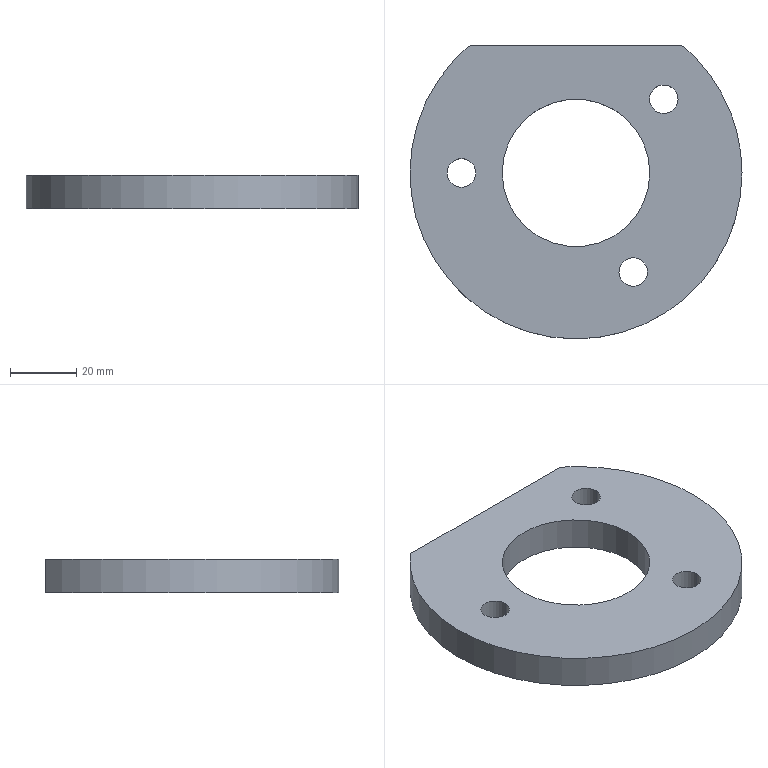Part | STEP file | 1_id1230_x_t | 1 solid | 12 faces | box 100 x 88.5 x 10 mm | volume 56263 mm3 | cylinder 9 | plane 3 | commonest cylinder face diameters 8.6 x6 44.45 x2 100 x1
STEP:
#1=CARTESIAN_POINT('',(0.,0.,0.));
#2=DIRECTION('',(0.,0.,1.));
#3=DIRECTION('',(1.,0.,0.));
#4=AXIS2_PLACEMENT_3D('',#1,#2,#3);
#5=CARTESIAN_POINT('',(112.925,347.5,90.11));
#6=VERTEX_POINT('',#5);
#7=CARTESIAN_POINT('',(31.023,386.,90.11));
#8=VERTEX_POINT('',#7);
#9=CARTESIAN_POINT('',(62.925,347.5,90.11));
#10=DIRECTION('',(0.,0.,-1.));
#11=DIRECTION('',(1.,0.,0.));
#12=AXIS2_PLACEMENT_3D('',#9,#10,#11);
#13=CIRCLE('',#12,50.);
#14=CARTESIAN_POINT('',(62.925,347.5,90.11));
#15=DIRECTION('',(0.,0.,1.));
#16=DIRECTION('',(1.,0.,0.));
#17=AXIS2_PLACEMENT_3D('',#14,#15,#16);
#18=PLANE('',#17);
#19=CARTESIAN_POINT('',(50.,0.));
#20=CARTESIAN_POINT('',(50.,-86.603));
#21=CARTESIAN_POINT('',(-25.,-43.301));
#22=CARTESIAN_POINT('',(-100.,0.));
#23=CARTESIAN_POINT('',(-25.,43.301));
#24=CARTESIAN_POINT('',(50.,86.603));
#25=CARTESIAN_POINT('',(50.,0.));
#26=(BOUNDED_CURVE()B_SPLINE_CURVE(2,(#19,#20,#21,#22,#23,#24,#25),.UNSPECIFIED.,.T.,.F.)B_SPLINE_CURVE_WITH_KNOTS((1,2,2,2,2,1),(-2.094,0.,2.094,4.189,6.283,8.378),.UNSPECIFIED.)CURVE()GEOMETRIC_REPRESENTATION_ITEM()RATIONAL_B_SPLINE_CURVE((1.,0.5,1.,0.5,1.,0.5,1.))REPRESENTATION_ITEM(''));
#27=(GEOMETRIC_REPRESENTATION_CONTEXT(2)PARAMETRIC_REPRESENTATION_CONTEXT()REPRESENTATION_CONTEXT('',''));
#28=DEFINITIONAL_REPRESENTATION('',(#26),#27);
#29=PCURVE('',#18,#28);
#30=CARTESIAN_POINT('',(62.925,347.5,100.11));
#31=DIRECTION('',(0.,0.,-1.));
#32=DIRECTION('',(-1.,0.,0.));
#33=AXIS2_PLACEMENT_3D('',#30,#31,#32);
#34=CYLINDRICAL_SURFACE('',#33,50.);
#35=CARTESIAN_POINT('',(3.142,10.));
#36=DIRECTION('',(1.,0.));
#37=VECTOR('',#36,1.);
#38=LINE('',#35,#37);
#39=(GEOMETRIC_REPRESENTATION_CONTEXT(2)PARAMETRIC_REPRESENTATION_CONTEXT()REPRESENTATION_CONTEXT('',''));
#40=DEFINITIONAL_REPRESENTATION('',(#38),#39);
#41=PCURVE('',#34,#40);
#42=SURFACE_CURVE('',#13,(#29,#41),.PCURVE_S1.);
#43=EDGE_CURVE('',#6,#8,#42,.T.);
#44=ORIENTED_EDGE('',*,*,#43,.T.);
#45=CARTESIAN_POINT('',(94.827,386.,90.11));
#46=VERTEX_POINT('',#45);
#47=CARTESIAN_POINT('',(94.827,386.,90.11));
#48=DIRECTION('',(-1.,0.,0.));
#49=VECTOR('',#48,1.);
#50=LINE('',#47,#49);
#51=CARTESIAN_POINT('',(31.902,38.5));
#52=DIRECTION('',(-1.,0.));
#53=VECTOR('',#52,1.);
#54=LINE('',#51,#53);
#55=(GEOMETRIC_REPRESENTATION_CONTEXT(2)PARAMETRIC_REPRESENTATION_CONTEXT()REPRESENTATION_CONTEXT('',''));
#56=DEFINITIONAL_REPRESENTATION('',(#54),#55);
#57=PCURVE('',#18,#56);
#58=CARTESIAN_POINT('',(167.925,386.,-58.465));
#59=DIRECTION('',(0.,-1.,0.));
#60=DIRECTION('',(0.,0.,1.));
#61=AXIS2_PLACEMENT_3D('',#58,#59,#60);
#62=PLANE('',#61);
#63=CARTESIAN_POINT('',(148.575,73.098));
#64=DIRECTION('',(0.,1.));
#65=VECTOR('',#64,1.);
#66=LINE('',#63,#65);
#67=(GEOMETRIC_REPRESENTATION_CONTEXT(2)PARAMETRIC_REPRESENTATION_CONTEXT()REPRESENTATION_CONTEXT('',''));
#68=DEFINITIONAL_REPRESENTATION('',(#66),#67);
#69=PCURVE('',#62,#68);
#70=SURFACE_CURVE('',#50,(#57,#69),.PCURVE_S1.);
#71=EDGE_CURVE('',#46,#8,#70,.T.);
#72=ORIENTED_EDGE('',*,*,#71,.F.);
#73=CARTESIAN_POINT('',(62.925,347.5,90.11));
#74=DIRECTION('',(0.,0.,-1.));
#75=DIRECTION('',(0.638,0.77,0.));
#76=AXIS2_PLACEMENT_3D('',#73,#74,#75);
#77=CIRCLE('',#76,50.);
#78=CARTESIAN_POINT('',(31.902,38.5));
#79=CARTESIAN_POINT('',(98.586,-16.756));
#80=CARTESIAN_POINT('',(17.391,-46.878));
#81=CARTESIAN_POINT('',(-63.804,-77.));
#82=CARTESIAN_POINT('',(-49.293,8.378));
#83=CARTESIAN_POINT('',(-34.782,93.756));
#84=CARTESIAN_POINT('',(31.902,38.5));
#85=(BOUNDED_CURVE()B_SPLINE_CURVE(2,(#78,#79,#80,#81,#82,#83,#84),.UNSPECIFIED.,.T.,.F.)B_SPLINE_CURVE_WITH_KNOTS((1,2,2,2,2,1),(-2.094,0.,2.094,4.189,6.283,8.378),.UNSPECIFIED.)CURVE()GEOMETRIC_REPRESENTATION_ITEM()RATIONAL_B_SPLINE_CURVE((1.,0.5,1.,0.5,1.,0.5,1.))REPRESENTATION_ITEM(''));
#86=(GEOMETRIC_REPRESENTATION_CONTEXT(2)PARAMETRIC_REPRESENTATION_CONTEXT()REPRESENTATION_CONTEXT('',''));
#87=DEFINITIONAL_REPRESENTATION('',(#85),#86);
#88=PCURVE('',#18,#87);
#89=CARTESIAN_POINT('',(2.263,10.));
#90=DIRECTION('',(1.,0.));
#91=VECTOR('',#90,1.);
#92=LINE('',#89,#91);
#93=(GEOMETRIC_REPRESENTATION_CONTEXT(2)PARAMETRIC_REPRESENTATION_CONTEXT()REPRESENTATION_CONTEXT('',''));
#94=DEFINITIONAL_REPRESENTATION('',(#92),#93);
#95=PCURVE('',#34,#94);
#96=SURFACE_CURVE('',#77,(#88,#95),.PCURVE_S1.);
#97=EDGE_CURVE('',#46,#6,#96,.T.);
#98=ORIENTED_EDGE('',*,*,#97,.T.);
#99=EDGE_LOOP('',(#44,#72,#98));
#100=FACE_BOUND('',#99,.T.);
#101=CARTESIAN_POINT('',(74.037,328.253,90.11));
#102=VERTEX_POINT('',#101);
#103=CARTESIAN_POINT('',(51.812,366.747,90.11));
#104=VERTEX_POINT('',#103);
#105=CARTESIAN_POINT('',(62.925,347.5,90.11));
#106=DIRECTION('',(0.,0.,1.));
#107=DIRECTION('',(0.5,-0.866,0.));
#108=AXIS2_PLACEMENT_3D('',#105,#106,#107);
#109=CIRCLE('',#108,22.225);
#110=CARTESIAN_POINT('',(0.,0.));
#111=DIRECTION('',(0.5,-0.866));
#112=AXIS2_PLACEMENT_2D('',#110,#111);
#113=CIRCLE('',#112,22.225);
#114=(GEOMETRIC_REPRESENTATION_CONTEXT(2)PARAMETRIC_REPRESENTATION_CONTEXT()REPRESENTATION_CONTEXT('',''));
#115=DEFINITIONAL_REPRESENTATION('',(#113),#114);
#116=PCURVE('',#18,#115);
#117=CARTESIAN_POINT('',(62.925,347.5,91.735));
#118=DIRECTION('',(0.,0.,1.));
#119=DIRECTION('',(-0.5,0.866,0.));
#120=AXIS2_PLACEMENT_3D('',#117,#118,#119);
#121=CYLINDRICAL_SURFACE('',#120,22.225);
#122=CARTESIAN_POINT('',(3.142,-1.625));
#123=DIRECTION('',(1.,0.));
#124=VECTOR('',#123,1.);
#125=LINE('',#122,#124);
#126=(GEOMETRIC_REPRESENTATION_CONTEXT(2)PARAMETRIC_REPRESENTATION_CONTEXT()REPRESENTATION_CONTEXT('',''));
#127=DEFINITIONAL_REPRESENTATION('',(#125),#126);
#128=PCURVE('',#121,#127);
#129=SURFACE_CURVE('',#109,(#116,#128),.PCURVE_S1.);
#130=EDGE_CURVE('',#102,#104,#129,.T.);
#131=ORIENTED_EDGE('',*,*,#130,.T.);
#132=CARTESIAN_POINT('',(40.7,347.5,90.11));
#133=VERTEX_POINT('',#132);
#134=CARTESIAN_POINT('',(62.925,347.5,90.11));
#135=DIRECTION('',(0.,0.,1.));
#136=DIRECTION('',(-0.5,0.866,0.));
#137=AXIS2_PLACEMENT_3D('',#134,#135,#136);
#138=CIRCLE('',#137,22.225);
#139=CARTESIAN_POINT('',(0.,0.));
#140=DIRECTION('',(-0.5,0.866));
#141=AXIS2_PLACEMENT_2D('',#139,#140);
#142=CIRCLE('',#141,22.225);
#143=(GEOMETRIC_REPRESENTATION_CONTEXT(2)PARAMETRIC_REPRESENTATION_CONTEXT()REPRESENTATION_CONTEXT('',''));
#144=DEFINITIONAL_REPRESENTATION('',(#142),#143);
#145=PCURVE('',#18,#144);
#146=CARTESIAN_POINT('',(62.925,347.5,91.735));
#147=DIRECTION('',(0.,0.,1.));
#148=DIRECTION('',(-0.5,0.866,0.));
#149=AXIS2_PLACEMENT_3D('',#146,#147,#148);
#150=CYLINDRICAL_SURFACE('',#149,22.225);
#151=CARTESIAN_POINT('',(0.,-1.625));
#152=DIRECTION('',(1.,0.));
#153=VECTOR('',#152,1.);
#154=LINE('',#151,#153);
#155=(GEOMETRIC_REPRESENTATION_CONTEXT(2)PARAMETRIC_REPRESENTATION_CONTEXT()REPRESENTATION_CONTEXT('',''));
#156=DEFINITIONAL_REPRESENTATION('',(#154),#155);
#157=PCURVE('',#150,#156);
#158=SURFACE_CURVE('',#138,(#145,#157),.PCURVE_S1.);
#159=EDGE_CURVE('',#104,#133,#158,.T.);
#160=ORIENTED_EDGE('',*,*,#159,.T.);
#161=CARTESIAN_POINT('',(62.925,347.5,90.11));
#162=DIRECTION('',(0.,0.,1.));
#163=DIRECTION('',(-1.,0.,0.));
#164=AXIS2_PLACEMENT_3D('',#161,#162,#163);
#165=CIRCLE('',#164,22.225);
#166=CARTESIAN_POINT('',(0.,0.));
#167=DIRECTION('',(-1.,0.));
#168=AXIS2_PLACEMENT_2D('',#166,#167);
#169=CIRCLE('',#168,22.225);
#170=(GEOMETRIC_REPRESENTATION_CONTEXT(2)PARAMETRIC_REPRESENTATION_CONTEXT()REPRESENTATION_CONTEXT('',''));
#171=DEFINITIONAL_REPRESENTATION('',(#169),#170);
#172=PCURVE('',#18,#171);
#173=CARTESIAN_POINT('',(1.047,-1.625));
#174=DIRECTION('',(1.,0.));
#175=VECTOR('',#174,1.);
#176=LINE('',#173,#175);
#177=(GEOMETRIC_REPRESENTATION_CONTEXT(2)PARAMETRIC_REPRESENTATION_CONTEXT()REPRESENTATION_CONTEXT('',''));
#178=DEFINITIONAL_REPRESENTATION('',(#176),#177);
#179=PCURVE('',#150,#178);
#180=SURFACE_CURVE('',#165,(#172,#179),.PCURVE_S1.);
#181=EDGE_CURVE('',#133,#102,#180,.T.);
#182=ORIENTED_EDGE('',*,*,#181,.T.);
#183=EDGE_LOOP('',(#131,#160,#182));
#184=FACE_BOUND('',#183,.T.);
#185=CARTESIAN_POINT('',(32.725,347.5,90.11));
#186=VERTEX_POINT('',#185);
#187=CARTESIAN_POINT('',(24.125,347.5,90.11));
#188=VERTEX_POINT('',#187);
#189=CARTESIAN_POINT('',(28.425,347.5,90.11));
#190=DIRECTION('',(0.,0.,1.));
#191=DIRECTION('',(1.,0.,0.));
#192=AXIS2_PLACEMENT_3D('',#189,#190,#191);
#193=CIRCLE('',#192,4.3);
#194=CARTESIAN_POINT('',(-34.5,0.));
#195=DIRECTION('',(1.,0.));
#196=AXIS2_PLACEMENT_2D('',#194,#195);
#197=CIRCLE('',#196,4.3);
#198=(GEOMETRIC_REPRESENTATION_CONTEXT(2)PARAMETRIC_REPRESENTATION_CONTEXT()REPRESENTATION_CONTEXT('',''));
#199=DEFINITIONAL_REPRESENTATION('',(#197),#198);
#200=PCURVE('',#18,#199);
#201=CARTESIAN_POINT('',(28.425,347.5,199.11));
#202=DIRECTION('',(0.,0.,-1.));
#203=DIRECTION('',(-1.,0.,0.));
#204=AXIS2_PLACEMENT_3D('',#201,#202,#203);
#205=CYLINDRICAL_SURFACE('',#204,4.3);
#206=CARTESIAN_POINT('',(3.142,109.));
#207=DIRECTION('',(-1.,0.));
#208=VECTOR('',#207,1.);
#209=LINE('',#206,#208);
#210=(GEOMETRIC_REPRESENTATION_CONTEXT(2)PARAMETRIC_REPRESENTATION_CONTEXT()REPRESENTATION_CONTEXT('',''));
#211=DEFINITIONAL_REPRESENTATION('',(#209),#210);
#212=PCURVE('',#205,#211);
#213=SURFACE_CURVE('',#193,(#200,#212),.PCURVE_S1.);
#214=EDGE_CURVE('',#186,#188,#213,.T.);
#215=ORIENTED_EDGE('',*,*,#214,.T.);
#216=CARTESIAN_POINT('',(28.425,347.5,90.11));
#217=DIRECTION('',(0.,0.,1.));
#218=DIRECTION('',(-1.,0.,0.));
#219=AXIS2_PLACEMENT_3D('',#216,#217,#218);
#220=CIRCLE('',#219,4.3);
#221=CARTESIAN_POINT('',(-34.5,0.));
#222=DIRECTION('',(-1.,0.));
#223=AXIS2_PLACEMENT_2D('',#221,#222);
#224=CIRCLE('',#223,4.3);
#225=(GEOMETRIC_REPRESENTATION_CONTEXT(2)PARAMETRIC_REPRESENTATION_CONTEXT()REPRESENTATION_CONTEXT('',''));
#226=DEFINITIONAL_REPRESENTATION('',(#224),#225);
#227=PCURVE('',#18,#226);
#228=CARTESIAN_POINT('',(28.425,347.5,199.11));
#229=DIRECTION('',(0.,0.,-1.));
#230=DIRECTION('',(-1.,0.,0.));
#231=AXIS2_PLACEMENT_3D('',#228,#229,#230);
#232=CYLINDRICAL_SURFACE('',#231,4.3);
#233=CARTESIAN_POINT('',(6.283,109.));
#234=DIRECTION('',(-1.,0.));
#235=VECTOR('',#234,1.);
#236=LINE('',#233,#235);
#237=(GEOMETRIC_REPRESENTATION_CONTEXT(2)PARAMETRIC_REPRESENTATION_CONTEXT()REPRESENTATION_CONTEXT('',''));
#238=DEFINITIONAL_REPRESENTATION('',(#236),#237);
#239=PCURVE('',#232,#238);
#240=SURFACE_CURVE('',#220,(#227,#239),.PCURVE_S1.);
#241=EDGE_CURVE('',#188,#186,#240,.T.);
#242=ORIENTED_EDGE('',*,*,#241,.T.);
#243=EDGE_LOOP('',(#215,#242));
#244=FACE_BOUND('',#243,.T.);
#245=CARTESIAN_POINT('',(93.654,369.676,90.11));
#246=VERTEX_POINT('',#245);
#247=CARTESIAN_POINT('',(85.054,369.676,90.11));
#248=VERTEX_POINT('',#247);
#249=CARTESIAN_POINT('',(89.354,369.676,90.11));
#250=DIRECTION('',(0.,0.,1.));
#251=DIRECTION('',(1.,0.,0.));
#252=AXIS2_PLACEMENT_3D('',#249,#250,#251);
#253=CIRCLE('',#252,4.3);
#254=CARTESIAN_POINT('',(26.429,22.176));
#255=DIRECTION('',(1.,0.));
#256=AXIS2_PLACEMENT_2D('',#254,#255);
#257=CIRCLE('',#256,4.3);
#258=(GEOMETRIC_REPRESENTATION_CONTEXT(2)PARAMETRIC_REPRESENTATION_CONTEXT()REPRESENTATION_CONTEXT('',''));
#259=DEFINITIONAL_REPRESENTATION('',(#257),#258);
#260=PCURVE('',#18,#259);
#261=CARTESIAN_POINT('',(89.354,369.676,199.11));
#262=DIRECTION('',(0.,0.,-1.));
#263=DIRECTION('',(-1.,0.,0.));
#264=AXIS2_PLACEMENT_3D('',#261,#262,#263);
#265=CYLINDRICAL_SURFACE('',#264,4.3);
#266=CARTESIAN_POINT('',(3.142,109.));
#267=DIRECTION('',(-1.,0.));
#268=VECTOR('',#267,1.);
#269=LINE('',#266,#268);
#270=(GEOMETRIC_REPRESENTATION_CONTEXT(2)PARAMETRIC_REPRESENTATION_CONTEXT()REPRESENTATION_CONTEXT('',''));
#271=DEFINITIONAL_REPRESENTATION('',(#269),#270);
#272=PCURVE('',#265,#271);
#273=SURFACE_CURVE('',#253,(#260,#272),.PCURVE_S1.);
#274=EDGE_CURVE('',#246,#248,#273,.T.);
#275=ORIENTED_EDGE('',*,*,#274,.T.);
#276=CARTESIAN_POINT('',(89.354,369.676,90.11));
#277=DIRECTION('',(0.,0.,1.));
#278=DIRECTION('',(-1.,0.,0.));
#279=AXIS2_PLACEMENT_3D('',#276,#277,#278);
#280=CIRCLE('',#279,4.3);
#281=CARTESIAN_POINT('',(26.429,22.176));
#282=DIRECTION('',(-1.,0.));
#283=AXIS2_PLACEMENT_2D('',#281,#282);
#284=CIRCLE('',#283,4.3);
#285=(GEOMETRIC_REPRESENTATION_CONTEXT(2)PARAMETRIC_REPRESENTATION_CONTEXT()REPRESENTATION_CONTEXT('',''));
#286=DEFINITIONAL_REPRESENTATION('',(#284),#285);
#287=PCURVE('',#18,#286);
#288=CARTESIAN_POINT('',(89.354,369.676,199.11));
#289=DIRECTION('',(0.,0.,-1.));
#290=DIRECTION('',(-1.,0.,0.));
#291=AXIS2_PLACEMENT_3D('',#288,#289,#290);
#292=CYLINDRICAL_SURFACE('',#291,4.3);
#293=CARTESIAN_POINT('',(6.283,109.));
#294=DIRECTION('',(-1.,0.));
#295=VECTOR('',#294,1.);
#296=LINE('',#293,#295);
#297=(GEOMETRIC_REPRESENTATION_CONTEXT(2)PARAMETRIC_REPRESENTATION_CONTEXT()REPRESENTATION_CONTEXT('',''));
#298=DEFINITIONAL_REPRESENTATION('',(#296),#297);
#299=PCURVE('',#292,#298);
#300=SURFACE_CURVE('',#280,(#287,#299),.PCURVE_S1.);
#301=EDGE_CURVE('',#248,#246,#300,.T.);
#302=ORIENTED_EDGE('',*,*,#301,.T.);
#303=EDGE_LOOP('',(#275,#302));
#304=FACE_BOUND('',#303,.T.);
#305=CARTESIAN_POINT('',(84.475,317.622,90.11));
#306=VERTEX_POINT('',#305);
#307=CARTESIAN_POINT('',(75.875,317.622,90.11));
#308=VERTEX_POINT('',#307);
#309=CARTESIAN_POINT('',(80.175,317.622,90.11));
#310=DIRECTION('',(0.,0.,1.));
#311=DIRECTION('',(1.,0.,0.));
#312=AXIS2_PLACEMENT_3D('',#309,#310,#311);
#313=CIRCLE('',#312,4.3);
#314=CARTESIAN_POINT('',(17.25,-29.878));
#315=DIRECTION('',(1.,0.));
#316=AXIS2_PLACEMENT_2D('',#314,#315);
#317=CIRCLE('',#316,4.3);
#318=(GEOMETRIC_REPRESENTATION_CONTEXT(2)PARAMETRIC_REPRESENTATION_CONTEXT()REPRESENTATION_CONTEXT('',''));
#319=DEFINITIONAL_REPRESENTATION('',(#317),#318);
#320=PCURVE('',#18,#319);
#321=CARTESIAN_POINT('',(80.175,317.622,199.11));
#322=DIRECTION('',(0.,0.,-1.));
#323=DIRECTION('',(-1.,0.,0.));
#324=AXIS2_PLACEMENT_3D('',#321,#322,#323);
#325=CYLINDRICAL_SURFACE('',#324,4.3);
#326=CARTESIAN_POINT('',(3.142,109.));
#327=DIRECTION('',(-1.,0.));
#328=VECTOR('',#327,1.);
#329=LINE('',#326,#328);
#330=(GEOMETRIC_REPRESENTATION_CONTEXT(2)PARAMETRIC_REPRESENTATION_CONTEXT()REPRESENTATION_CONTEXT('',''));
#331=DEFINITIONAL_REPRESENTATION('',(#329),#330);
#332=PCURVE('',#325,#331);
#333=SURFACE_CURVE('',#313,(#320,#332),.PCURVE_S1.);
#334=EDGE_CURVE('',#306,#308,#333,.T.);
#335=ORIENTED_EDGE('',*,*,#334,.T.);
#336=CARTESIAN_POINT('',(80.175,317.622,90.11));
#337=DIRECTION('',(0.,0.,1.));
#338=DIRECTION('',(-1.,0.,0.));
#339=AXIS2_PLACEMENT_3D('',#336,#337,#338);
#340=CIRCLE('',#339,4.3);
#341=CARTESIAN_POINT('',(17.25,-29.878));
#342=DIRECTION('',(-1.,0.));
#343=AXIS2_PLACEMENT_2D('',#341,#342);
#344=CIRCLE('',#343,4.3);
#345=(GEOMETRIC_REPRESENTATION_CONTEXT(2)PARAMETRIC_REPRESENTATION_CONTEXT()REPRESENTATION_CONTEXT('',''));
#346=DEFINITIONAL_REPRESENTATION('',(#344),#345);
#347=PCURVE('',#18,#346);
#348=CARTESIAN_POINT('',(80.175,317.622,199.11));
#349=DIRECTION('',(0.,0.,-1.));
#350=DIRECTION('',(-1.,0.,0.));
#351=AXIS2_PLACEMENT_3D('',#348,#349,#350);
#352=CYLINDRICAL_SURFACE('',#351,4.3);
#353=CARTESIAN_POINT('',(6.283,109.));
#354=DIRECTION('',(-1.,0.));
#355=VECTOR('',#354,1.);
#356=LINE('',#353,#355);
#357=(GEOMETRIC_REPRESENTATION_CONTEXT(2)PARAMETRIC_REPRESENTATION_CONTEXT()REPRESENTATION_CONTEXT('',''));
#358=DEFINITIONAL_REPRESENTATION('',(#356),#357);
#359=PCURVE('',#352,#358);
#360=SURFACE_CURVE('',#340,(#347,#359),.PCURVE_S1.);
#361=EDGE_CURVE('',#308,#306,#360,.T.);
#362=ORIENTED_EDGE('',*,*,#361,.T.);
#363=EDGE_LOOP('',(#335,#362));
#364=FACE_BOUND('',#363,.T.);
#365=ADVANCED_FACE('',(#100,#184,#244,#304,#364),#18,.F.);
#366=CARTESIAN_POINT('',(74.037,328.253,100.11));
#367=VERTEX_POINT('',#366);
#368=CARTESIAN_POINT('',(40.7,347.5,100.11));
#369=VERTEX_POINT('',#368);
#370=CARTESIAN_POINT('',(62.925,347.5,100.11));
#371=DIRECTION('',(0.,0.,-1.));
#372=DIRECTION('',(0.5,-0.866,0.));
#373=AXIS2_PLACEMENT_3D('',#370,#371,#372);
#374=CIRCLE('',#373,22.225);
#375=CARTESIAN_POINT('',(3.142,8.375));
#376=DIRECTION('',(-1.,0.));
#377=VECTOR('',#376,1.);
#378=LINE('',#375,#377);
#379=(GEOMETRIC_REPRESENTATION_CONTEXT(2)PARAMETRIC_REPRESENTATION_CONTEXT()REPRESENTATION_CONTEXT('',''));
#380=DEFINITIONAL_REPRESENTATION('',(#378),#379);
#381=PCURVE('',#150,#380);
#382=CARTESIAN_POINT('',(62.925,347.5,100.11));
#383=DIRECTION('',(0.,0.,1.));
#384=DIRECTION('',(1.,0.,0.));
#385=AXIS2_PLACEMENT_3D('',#382,#383,#384);
#386=PLANE('',#385);
#387=CARTESIAN_POINT('',(11.113,-19.247));
#388=CARTESIAN_POINT('',(-22.225,-38.495));
#389=CARTESIAN_POINT('',(-22.225,0.));
#390=CARTESIAN_POINT('',(-22.225,38.495));
#391=CARTESIAN_POINT('',(11.113,19.247));
#392=CARTESIAN_POINT('',(44.45,0.));
#393=CARTESIAN_POINT('',(11.113,-19.247));
#394=(BOUNDED_CURVE()B_SPLINE_CURVE(2,(#387,#388,#389,#390,#391,#392,#393),.UNSPECIFIED.,.T.,.F.)B_SPLINE_CURVE_WITH_KNOTS((1,2,2,2,2,1),(-2.094,0.,2.094,4.189,6.283,8.378),.UNSPECIFIED.)CURVE()GEOMETRIC_REPRESENTATION_ITEM()RATIONAL_B_SPLINE_CURVE((1.,0.5,1.,0.5,1.,0.5,1.))REPRESENTATION_ITEM(''));
#395=(GEOMETRIC_REPRESENTATION_CONTEXT(2)PARAMETRIC_REPRESENTATION_CONTEXT()REPRESENTATION_CONTEXT('',''));
#396=DEFINITIONAL_REPRESENTATION('',(#394),#395);
#397=PCURVE('',#386,#396);
#398=SURFACE_CURVE('',#374,(#381,#397),.PCURVE_S1.);
#399=EDGE_CURVE('',#367,#369,#398,.T.);
#400=ORIENTED_EDGE('',*,*,#399,.T.);
#401=CARTESIAN_POINT('',(51.812,366.747,100.11));
#402=VERTEX_POINT('',#401);
#403=CARTESIAN_POINT('',(62.925,347.5,100.11));
#404=DIRECTION('',(0.,0.,-1.));
#405=DIRECTION('',(-1.,0.,0.));
#406=AXIS2_PLACEMENT_3D('',#403,#404,#405);
#407=CIRCLE('',#406,22.225);
#408=CARTESIAN_POINT('',(1.047,8.375));
#409=DIRECTION('',(-1.,0.));
#410=VECTOR('',#409,1.);
#411=LINE('',#408,#410);
#412=(GEOMETRIC_REPRESENTATION_CONTEXT(2)PARAMETRIC_REPRESENTATION_CONTEXT()REPRESENTATION_CONTEXT('',''));
#413=DEFINITIONAL_REPRESENTATION('',(#411),#412);
#414=PCURVE('',#150,#413);
#415=CARTESIAN_POINT('',(-22.225,0.));
#416=CARTESIAN_POINT('',(-22.225,38.495));
#417=CARTESIAN_POINT('',(11.113,19.247));
#418=CARTESIAN_POINT('',(44.45,0.));
#419=CARTESIAN_POINT('',(11.113,-19.247));
#420=CARTESIAN_POINT('',(-22.225,-38.495));
#421=CARTESIAN_POINT('',(-22.225,0.));
#422=(BOUNDED_CURVE()B_SPLINE_CURVE(2,(#415,#416,#417,#418,#419,#420,#421),.UNSPECIFIED.,.T.,.F.)B_SPLINE_CURVE_WITH_KNOTS((1,2,2,2,2,1),(-2.094,0.,2.094,4.189,6.283,8.378),.UNSPECIFIED.)CURVE()GEOMETRIC_REPRESENTATION_ITEM()RATIONAL_B_SPLINE_CURVE((1.,0.5,1.,0.5,1.,0.5,1.))REPRESENTATION_ITEM(''));
#423=(GEOMETRIC_REPRESENTATION_CONTEXT(2)PARAMETRIC_REPRESENTATION_CONTEXT()REPRESENTATION_CONTEXT('',''));
#424=DEFINITIONAL_REPRESENTATION('',(#422),#423);
#425=PCURVE('',#386,#424);
#426=SURFACE_CURVE('',#407,(#414,#425),.PCURVE_S1.);
#427=EDGE_CURVE('',#369,#402,#426,.T.);
#428=ORIENTED_EDGE('',*,*,#427,.T.);
#429=CARTESIAN_POINT('',(51.812,366.747,90.11));
#430=DIRECTION('',(0.,0.,1.));
#431=VECTOR('',#430,1.);
#432=LINE('',#429,#431);
#433=CARTESIAN_POINT('',(0.,-1.625));
#434=DIRECTION('',(0.,1.));
#435=VECTOR('',#434,1.);
#436=LINE('',#433,#435);
#437=(GEOMETRIC_REPRESENTATION_CONTEXT(2)PARAMETRIC_REPRESENTATION_CONTEXT()REPRESENTATION_CONTEXT('',''));
#438=DEFINITIONAL_REPRESENTATION('',(#436),#437);
#439=PCURVE('',#150,#438);
#440=CARTESIAN_POINT('',(6.283,-1.625));
#441=DIRECTION('',(0.,1.));
#442=VECTOR('',#441,1.);
#443=LINE('',#440,#442);
#444=(GEOMETRIC_REPRESENTATION_CONTEXT(2)PARAMETRIC_REPRESENTATION_CONTEXT()REPRESENTATION_CONTEXT('',''));
#445=DEFINITIONAL_REPRESENTATION('',(#443),#444);
#446=PCURVE('',#121,#445);
#447=SURFACE_CURVE('',#432,(#439,#446),.PCURVE_S1.);
#448=EDGE_CURVE('',#104,#402,#447,.T.);
#449=ORIENTED_EDGE('',*,*,#448,.F.);
#450=ORIENTED_EDGE('',*,*,#159,.T.);
#451=ORIENTED_EDGE('',*,*,#181,.T.);
#452=CARTESIAN_POINT('',(74.037,328.253,90.11));
#453=DIRECTION('',(0.,0.,-1.));
#454=VECTOR('',#453,1.);
#455=LINE('',#452,#454);
#456=CARTESIAN_POINT('',(3.142,-1.625));
#457=DIRECTION('',(0.,-1.));
#458=VECTOR('',#457,1.);
#459=LINE('',#456,#458);
#460=(GEOMETRIC_REPRESENTATION_CONTEXT(2)PARAMETRIC_REPRESENTATION_CONTEXT()REPRESENTATION_CONTEXT('',''));
#461=DEFINITIONAL_REPRESENTATION('',(#459),#460);
#462=PCURVE('',#150,#461);
#463=CARTESIAN_POINT('',(3.142,-1.625));
#464=DIRECTION('',(0.,-1.));
#465=VECTOR('',#464,1.);
#466=LINE('',#463,#465);
#467=(GEOMETRIC_REPRESENTATION_CONTEXT(2)PARAMETRIC_REPRESENTATION_CONTEXT()REPRESENTATION_CONTEXT('',''));
#468=DEFINITIONAL_REPRESENTATION('',(#466),#467);
#469=PCURVE('',#121,#468);
#470=SURFACE_CURVE('',#455,(#462,#469),.PCURVE_S1.);
#471=EDGE_CURVE('',#367,#102,#470,.T.);
#472=ORIENTED_EDGE('',*,*,#471,.F.);
#473=EDGE_LOOP('',(#400,#428,#449,#450,#451,#472));
#474=FACE_BOUND('',#473,.F.);
#475=ADVANCED_FACE('',(#474),#150,.F.);
#476=CARTESIAN_POINT('',(31.023,386.,100.11));
#477=VERTEX_POINT('',#476);
#478=CARTESIAN_POINT('',(112.925,347.5,100.11));
#479=VERTEX_POINT('',#478);
#480=CARTESIAN_POINT('',(62.925,347.5,100.11));
#481=DIRECTION('',(0.,0.,1.));
#482=DIRECTION('',(-0.638,0.77,0.));
#483=AXIS2_PLACEMENT_3D('',#480,#481,#482);
#484=CIRCLE('',#483,50.);
#485=CARTESIAN_POINT('',(0.,0.));
#486=DIRECTION('',(-0.638,0.77));
#487=AXIS2_PLACEMENT_2D('',#485,#486);
#488=CIRCLE('',#487,50.);
#489=(GEOMETRIC_REPRESENTATION_CONTEXT(2)PARAMETRIC_REPRESENTATION_CONTEXT()REPRESENTATION_CONTEXT('',''));
#490=DEFINITIONAL_REPRESENTATION('',(#488),#489);
#491=PCURVE('',#386,#490);
#492=CARTESIAN_POINT('',(7.162,0.));
#493=DIRECTION('',(-1.,0.));
#494=VECTOR('',#493,1.);
#495=LINE('',#492,#494);
#496=(GEOMETRIC_REPRESENTATION_CONTEXT(2)PARAMETRIC_REPRESENTATION_CONTEXT()REPRESENTATION_CONTEXT('',''));
#497=DEFINITIONAL_REPRESENTATION('',(#495),#496);
#498=PCURVE('',#34,#497);
#499=SURFACE_CURVE('',#484,(#491,#498),.PCURVE_S1.);
#500=EDGE_CURVE('',#477,#479,#499,.T.);
#501=ORIENTED_EDGE('',*,*,#500,.T.);
#502=CARTESIAN_POINT('',(94.827,386.,100.11));
#503=VERTEX_POINT('',#502);
#504=CARTESIAN_POINT('',(62.925,347.5,100.11));
#505=DIRECTION('',(0.,0.,1.));
#506=DIRECTION('',(1.,0.,0.));
#507=AXIS2_PLACEMENT_3D('',#504,#505,#506);
#508=CIRCLE('',#507,50.);
#509=CARTESIAN_POINT('',(0.,0.));
#510=DIRECTION('',(1.,0.));
#511=AXIS2_PLACEMENT_2D('',#509,#510);
#512=CIRCLE('',#511,50.);
#513=(GEOMETRIC_REPRESENTATION_CONTEXT(2)PARAMETRIC_REPRESENTATION_CONTEXT()REPRESENTATION_CONTEXT('',''));
#514=DEFINITIONAL_REPRESENTATION('',(#512),#513);
#515=PCURVE('',#386,#514);
#516=CARTESIAN_POINT('',(3.142,0.));
#517=DIRECTION('',(-1.,0.));
#518=VECTOR('',#517,1.);
#519=LINE('',#516,#518);
#520=(GEOMETRIC_REPRESENTATION_CONTEXT(2)PARAMETRIC_REPRESENTATION_CONTEXT()REPRESENTATION_CONTEXT('',''));
#521=DEFINITIONAL_REPRESENTATION('',(#519),#520);
#522=PCURVE('',#34,#521);
#523=SURFACE_CURVE('',#508,(#515,#522),.PCURVE_S1.);
#524=EDGE_CURVE('',#479,#503,#523,.T.);
#525=ORIENTED_EDGE('',*,*,#524,.T.);
#526=CARTESIAN_POINT('',(94.827,386.,100.11));
#527=DIRECTION('',(-1.,0.,0.));
#528=VECTOR('',#527,1.);
#529=LINE('',#526,#528);
#530=CARTESIAN_POINT('',(31.902,38.5));
#531=DIRECTION('',(-1.,0.));
#532=VECTOR('',#531,1.);
#533=LINE('',#530,#532);
#534=(GEOMETRIC_REPRESENTATION_CONTEXT(2)PARAMETRIC_REPRESENTATION_CONTEXT()REPRESENTATION_CONTEXT('',''));
#535=DEFINITIONAL_REPRESENTATION('',(#533),#534);
#536=PCURVE('',#386,#535);
#537=CARTESIAN_POINT('',(158.575,73.098));
#538=DIRECTION('',(0.,1.));
#539=VECTOR('',#538,1.);
#540=LINE('',#537,#539);
#541=(GEOMETRIC_REPRESENTATION_CONTEXT(2)PARAMETRIC_REPRESENTATION_CONTEXT()REPRESENTATION_CONTEXT('',''));
#542=DEFINITIONAL_REPRESENTATION('',(#540),#541);
#543=PCURVE('',#62,#542);
#544=SURFACE_CURVE('',#529,(#536,#543),.PCURVE_S1.);
#545=EDGE_CURVE('',#503,#477,#544,.T.);
#546=ORIENTED_EDGE('',*,*,#545,.T.);
#547=EDGE_LOOP('',(#501,#525,#546));
#548=FACE_BOUND('',#547,.T.);
#549=CARTESIAN_POINT('',(32.725,347.5,100.11));
#550=VERTEX_POINT('',#549);
#551=CARTESIAN_POINT('',(24.125,347.5,100.11));
#552=VERTEX_POINT('',#551);
#553=CARTESIAN_POINT('',(28.425,347.5,100.11));
#554=DIRECTION('',(0.,0.,-1.));
#555=DIRECTION('',(1.,0.,0.));
#556=AXIS2_PLACEMENT_3D('',#553,#554,#555);
#557=CIRCLE('',#556,4.3);
#558=CARTESIAN_POINT('',(-30.2,0.));
#559=CARTESIAN_POINT('',(-30.2,-7.448));
#560=CARTESIAN_POINT('',(-36.65,-3.724));
#561=CARTESIAN_POINT('',(-43.1,0.));
#562=CARTESIAN_POINT('',(-36.65,3.724));
#563=CARTESIAN_POINT('',(-30.2,7.448));
#564=CARTESIAN_POINT('',(-30.2,0.));
#565=(BOUNDED_CURVE()B_SPLINE_CURVE(2,(#558,#559,#560,#561,#562,#563,#564),.UNSPECIFIED.,.T.,.F.)B_SPLINE_CURVE_WITH_KNOTS((1,2,2,2,2,1),(-2.094,0.,2.094,4.189,6.283,8.378),.UNSPECIFIED.)CURVE()GEOMETRIC_REPRESENTATION_ITEM()RATIONAL_B_SPLINE_CURVE((1.,0.5,1.,0.5,1.,0.5,1.))REPRESENTATION_ITEM(''));
#566=(GEOMETRIC_REPRESENTATION_CONTEXT(2)PARAMETRIC_REPRESENTATION_CONTEXT()REPRESENTATION_CONTEXT('',''));
#567=DEFINITIONAL_REPRESENTATION('',(#565),#566);
#568=PCURVE('',#386,#567);
#569=CARTESIAN_POINT('',(3.142,99.));
#570=DIRECTION('',(1.,0.));
#571=VECTOR('',#570,1.);
#572=LINE('',#569,#571);
#573=(GEOMETRIC_REPRESENTATION_CONTEXT(2)PARAMETRIC_REPRESENTATION_CONTEXT()REPRESENTATION_CONTEXT('',''));
#574=DEFINITIONAL_REPRESENTATION('',(#572),#573);
#575=PCURVE('',#232,#574);
#576=SURFACE_CURVE('',#557,(#568,#575),.PCURVE_S1.);
#577=EDGE_CURVE('',#550,#552,#576,.T.);
#578=ORIENTED_EDGE('',*,*,#577,.T.);
#579=CARTESIAN_POINT('',(28.425,347.5,100.11));
#580=DIRECTION('',(0.,0.,-1.));
#581=DIRECTION('',(-1.,0.,0.));
#582=AXIS2_PLACEMENT_3D('',#579,#580,#581);
#583=CIRCLE('',#582,4.3);
#584=CARTESIAN_POINT('',(-38.8,0.));
#585=CARTESIAN_POINT('',(-38.8,7.448));
#586=CARTESIAN_POINT('',(-32.35,3.724));
#587=CARTESIAN_POINT('',(-25.9,0.));
#588=CARTESIAN_POINT('',(-32.35,-3.724));
#589=CARTESIAN_POINT('',(-38.8,-7.448));
#590=CARTESIAN_POINT('',(-38.8,0.));
#591=(BOUNDED_CURVE()B_SPLINE_CURVE(2,(#584,#585,#586,#587,#588,#589,#590),.UNSPECIFIED.,.T.,.F.)B_SPLINE_CURVE_WITH_KNOTS((1,2,2,2,2,1),(-2.094,0.,2.094,4.189,6.283,8.378),.UNSPECIFIED.)CURVE()GEOMETRIC_REPRESENTATION_ITEM()RATIONAL_B_SPLINE_CURVE((1.,0.5,1.,0.5,1.,0.5,1.))REPRESENTATION_ITEM(''));
#592=(GEOMETRIC_REPRESENTATION_CONTEXT(2)PARAMETRIC_REPRESENTATION_CONTEXT()REPRESENTATION_CONTEXT('',''));
#593=DEFINITIONAL_REPRESENTATION('',(#591),#592);
#594=PCURVE('',#386,#593);
#595=CARTESIAN_POINT('',(0.,99.));
#596=DIRECTION('',(1.,0.));
#597=VECTOR('',#596,1.);
#598=LINE('',#595,#597);
#599=(GEOMETRIC_REPRESENTATION_CONTEXT(2)PARAMETRIC_REPRESENTATION_CONTEXT()REPRESENTATION_CONTEXT('',''));
#600=DEFINITIONAL_REPRESENTATION('',(#598),#599);
#601=PCURVE('',#205,#600);
#602=SURFACE_CURVE('',#583,(#594,#601),.PCURVE_S1.);
#603=EDGE_CURVE('',#552,#550,#602,.T.);
#604=ORIENTED_EDGE('',*,*,#603,.T.);
#605=EDGE_LOOP('',(#578,#604));
#606=FACE_BOUND('',#605,.T.);
#607=CARTESIAN_POINT('',(93.654,369.676,100.11));
#608=VERTEX_POINT('',#607);
#609=CARTESIAN_POINT('',(85.054,369.676,100.11));
#610=VERTEX_POINT('',#609);
#611=CARTESIAN_POINT('',(89.354,369.676,100.11));
#612=DIRECTION('',(0.,0.,-1.));
#613=DIRECTION('',(1.,0.,0.));
#614=AXIS2_PLACEMENT_3D('',#611,#612,#613);
#615=CIRCLE('',#614,4.3);
#616=CARTESIAN_POINT('',(30.729,22.176));
#617=CARTESIAN_POINT('',(30.729,14.728));
#618=CARTESIAN_POINT('',(24.279,18.452));
#619=CARTESIAN_POINT('',(17.829,22.176));
#620=CARTESIAN_POINT('',(24.279,25.9));
#621=CARTESIAN_POINT('',(30.729,29.624));
#622=CARTESIAN_POINT('',(30.729,22.176));
#623=(BOUNDED_CURVE()B_SPLINE_CURVE(2,(#616,#617,#618,#619,#620,#621,#622),.UNSPECIFIED.,.T.,.F.)B_SPLINE_CURVE_WITH_KNOTS((1,2,2,2,2,1),(-2.094,0.,2.094,4.189,6.283,8.378),.UNSPECIFIED.)CURVE()GEOMETRIC_REPRESENTATION_ITEM()RATIONAL_B_SPLINE_CURVE((1.,0.5,1.,0.5,1.,0.5,1.))REPRESENTATION_ITEM(''));
#624=(GEOMETRIC_REPRESENTATION_CONTEXT(2)PARAMETRIC_REPRESENTATION_CONTEXT()REPRESENTATION_CONTEXT('',''));
#625=DEFINITIONAL_REPRESENTATION('',(#623),#624);
#626=PCURVE('',#386,#625);
#627=CARTESIAN_POINT('',(3.142,99.));
#628=DIRECTION('',(1.,0.));
#629=VECTOR('',#628,1.);
#630=LINE('',#627,#629);
#631=(GEOMETRIC_REPRESENTATION_CONTEXT(2)PARAMETRIC_REPRESENTATION_CONTEXT()REPRESENTATION_CONTEXT('',''));
#632=DEFINITIONAL_REPRESENTATION('',(#630),#631);
#633=PCURVE('',#292,#632);
#634=SURFACE_CURVE('',#615,(#626,#633),.PCURVE_S1.);
#635=EDGE_CURVE('',#608,#610,#634,.T.);
#636=ORIENTED_EDGE('',*,*,#635,.T.);
#637=CARTESIAN_POINT('',(89.354,369.676,100.11));
#638=DIRECTION('',(0.,0.,-1.));
#639=DIRECTION('',(-1.,0.,0.));
#640=AXIS2_PLACEMENT_3D('',#637,#638,#639);
#641=CIRCLE('',#640,4.3);
#642=CARTESIAN_POINT('',(22.129,22.176));
#643=CARTESIAN_POINT('',(22.129,29.624));
#644=CARTESIAN_POINT('',(28.579,25.9));
#645=CARTESIAN_POINT('',(35.029,22.176));
#646=CARTESIAN_POINT('',(28.579,18.452));
#647=CARTESIAN_POINT('',(22.129,14.728));
#648=CARTESIAN_POINT('',(22.129,22.176));
#649=(BOUNDED_CURVE()B_SPLINE_CURVE(2,(#642,#643,#644,#645,#646,#647,#648),.UNSPECIFIED.,.T.,.F.)B_SPLINE_CURVE_WITH_KNOTS((1,2,2,2,2,1),(-2.094,0.,2.094,4.189,6.283,8.378),.UNSPECIFIED.)CURVE()GEOMETRIC_REPRESENTATION_ITEM()RATIONAL_B_SPLINE_CURVE((1.,0.5,1.,0.5,1.,0.5,1.))REPRESENTATION_ITEM(''));
#650=(GEOMETRIC_REPRESENTATION_CONTEXT(2)PARAMETRIC_REPRESENTATION_CONTEXT()REPRESENTATION_CONTEXT('',''));
#651=DEFINITIONAL_REPRESENTATION('',(#649),#650);
#652=PCURVE('',#386,#651);
#653=CARTESIAN_POINT('',(0.,99.));
#654=DIRECTION('',(1.,0.));
#655=VECTOR('',#654,1.);
#656=LINE('',#653,#655);
#657=(GEOMETRIC_REPRESENTATION_CONTEXT(2)PARAMETRIC_REPRESENTATION_CONTEXT()REPRESENTATION_CONTEXT('',''));
#658=DEFINITIONAL_REPRESENTATION('',(#656),#657);
#659=PCURVE('',#265,#658);
#660=SURFACE_CURVE('',#641,(#652,#659),.PCURVE_S1.);
#661=EDGE_CURVE('',#610,#608,#660,.T.);
#662=ORIENTED_EDGE('',*,*,#661,.T.);
#663=EDGE_LOOP('',(#636,#662));
#664=FACE_BOUND('',#663,.T.);
#665=CARTESIAN_POINT('',(84.475,317.622,100.11));
#666=VERTEX_POINT('',#665);
#667=CARTESIAN_POINT('',(75.875,317.622,100.11));
#668=VERTEX_POINT('',#667);
#669=CARTESIAN_POINT('',(80.175,317.622,100.11));
#670=DIRECTION('',(0.,0.,-1.));
#671=DIRECTION('',(1.,0.,0.));
#672=AXIS2_PLACEMENT_3D('',#669,#670,#671);
#673=CIRCLE('',#672,4.3);
#674=CARTESIAN_POINT('',(21.55,-29.878));
#675=CARTESIAN_POINT('',(21.55,-37.326));
#676=CARTESIAN_POINT('',(15.1,-33.602));
#677=CARTESIAN_POINT('',(8.65,-29.878));
#678=CARTESIAN_POINT('',(15.1,-26.154));
#679=CARTESIAN_POINT('',(21.55,-22.43));
#680=CARTESIAN_POINT('',(21.55,-29.878));
#681=(BOUNDED_CURVE()B_SPLINE_CURVE(2,(#674,#675,#676,#677,#678,#679,#680),.UNSPECIFIED.,.T.,.F.)B_SPLINE_CURVE_WITH_KNOTS((1,2,2,2,2,1),(-2.094,0.,2.094,4.189,6.283,8.378),.UNSPECIFIED.)CURVE()GEOMETRIC_REPRESENTATION_ITEM()RATIONAL_B_SPLINE_CURVE((1.,0.5,1.,0.5,1.,0.5,1.))REPRESENTATION_ITEM(''));
#682=(GEOMETRIC_REPRESENTATION_CONTEXT(2)PARAMETRIC_REPRESENTATION_CONTEXT()REPRESENTATION_CONTEXT('',''));
#683=DEFINITIONAL_REPRESENTATION('',(#681),#682);
#684=PCURVE('',#386,#683);
#685=CARTESIAN_POINT('',(3.142,99.));
#686=DIRECTION('',(1.,0.));
#687=VECTOR('',#686,1.);
#688=LINE('',#685,#687);
#689=(GEOMETRIC_REPRESENTATION_CONTEXT(2)PARAMETRIC_REPRESENTATION_CONTEXT()REPRESENTATION_CONTEXT('',''));
#690=DEFINITIONAL_REPRESENTATION('',(#688),#689);
#691=PCURVE('',#352,#690);
#692=SURFACE_CURVE('',#673,(#684,#691),.PCURVE_S1.);
#693=EDGE_CURVE('',#666,#668,#692,.T.);
#694=ORIENTED_EDGE('',*,*,#693,.T.);
#695=CARTESIAN_POINT('',(80.175,317.622,100.11));
#696=DIRECTION('',(0.,0.,-1.));
#697=DIRECTION('',(-1.,0.,0.));
#698=AXIS2_PLACEMENT_3D('',#695,#696,#697);
#699=CIRCLE('',#698,4.3);
#700=CARTESIAN_POINT('',(12.95,-29.878));
#701=CARTESIAN_POINT('',(12.95,-22.43));
#702=CARTESIAN_POINT('',(19.4,-26.154));
#703=CARTESIAN_POINT('',(25.85,-29.878));
#704=CARTESIAN_POINT('',(19.4,-33.602));
#705=CARTESIAN_POINT('',(12.95,-37.326));
#706=CARTESIAN_POINT('',(12.95,-29.878));
#707=(BOUNDED_CURVE()B_SPLINE_CURVE(2,(#700,#701,#702,#703,#704,#705,#706),.UNSPECIFIED.,.T.,.F.)B_SPLINE_CURVE_WITH_KNOTS((1,2,2,2,2,1),(-2.094,0.,2.094,4.189,6.283,8.378),.UNSPECIFIED.)CURVE()GEOMETRIC_REPRESENTATION_ITEM()RATIONAL_B_SPLINE_CURVE((1.,0.5,1.,0.5,1.,0.5,1.))REPRESENTATION_ITEM(''));
#708=(GEOMETRIC_REPRESENTATION_CONTEXT(2)PARAMETRIC_REPRESENTATION_CONTEXT()REPRESENTATION_CONTEXT('',''));
#709=DEFINITIONAL_REPRESENTATION('',(#707),#708);
#710=PCURVE('',#386,#709);
#711=CARTESIAN_POINT('',(0.,99.));
#712=DIRECTION('',(1.,0.));
#713=VECTOR('',#712,1.);
#714=LINE('',#711,#713);
#715=(GEOMETRIC_REPRESENTATION_CONTEXT(2)PARAMETRIC_REPRESENTATION_CONTEXT()REPRESENTATION_CONTEXT('',''));
#716=DEFINITIONAL_REPRESENTATION('',(#714),#715);
#717=PCURVE('',#325,#716);
#718=SURFACE_CURVE('',#699,(#710,#717),.PCURVE_S1.);
#719=EDGE_CURVE('',#668,#666,#718,.T.);
#720=ORIENTED_EDGE('',*,*,#719,.T.);
#721=EDGE_LOOP('',(#694,#720));
#722=FACE_BOUND('',#721,.T.);
#723=CARTESIAN_POINT('',(62.925,347.5,100.11));
#724=DIRECTION('',(0.,0.,-1.));
#725=DIRECTION('',(-0.5,0.866,0.));
#726=AXIS2_PLACEMENT_3D('',#723,#724,#725);
#727=CIRCLE('',#726,22.225);
#728=CARTESIAN_POINT('',(-11.113,19.247));
#729=CARTESIAN_POINT('',(22.225,38.495));
#730=CARTESIAN_POINT('',(22.225,0.));
#731=CARTESIAN_POINT('',(22.225,-38.495));
#732=CARTESIAN_POINT('',(-11.113,-19.247));
#733=CARTESIAN_POINT('',(-44.45,0.));
#734=CARTESIAN_POINT('',(-11.113,19.247));
#735=(BOUNDED_CURVE()B_SPLINE_CURVE(2,(#728,#729,#730,#731,#732,#733,#734),.UNSPECIFIED.,.T.,.F.)B_SPLINE_CURVE_WITH_KNOTS((1,2,2,2,2,1),(-2.094,0.,2.094,4.189,6.283,8.378),.UNSPECIFIED.)CURVE()GEOMETRIC_REPRESENTATION_ITEM()RATIONAL_B_SPLINE_CURVE((1.,0.5,1.,0.5,1.,0.5,1.))REPRESENTATION_ITEM(''));
#736=(GEOMETRIC_REPRESENTATION_CONTEXT(2)PARAMETRIC_REPRESENTATION_CONTEXT()REPRESENTATION_CONTEXT('',''));
#737=DEFINITIONAL_REPRESENTATION('',(#735),#736);
#738=PCURVE('',#386,#737);
#739=CARTESIAN_POINT('',(6.283,8.375));
#740=DIRECTION('',(-1.,0.));
#741=VECTOR('',#740,1.);
#742=LINE('',#739,#741);
#743=(GEOMETRIC_REPRESENTATION_CONTEXT(2)PARAMETRIC_REPRESENTATION_CONTEXT()REPRESENTATION_CONTEXT('',''));
#744=DEFINITIONAL_REPRESENTATION('',(#742),#743);
#745=PCURVE('',#121,#744);
#746=SURFACE_CURVE('',#727,(#738,#745),.PCURVE_S1.);
#747=EDGE_CURVE('',#402,#367,#746,.T.);
#748=ORIENTED_EDGE('',*,*,#747,.T.);
#749=ORIENTED_EDGE('',*,*,#399,.T.);
#750=ORIENTED_EDGE('',*,*,#427,.T.);
#751=EDGE_LOOP('',(#748,#749,#750));
#752=FACE_BOUND('',#751,.T.);
#753=ADVANCED_FACE('',(#548,#606,#664,#722,#752),#386,.T.);
#754=ORIENTED_EDGE('',*,*,#603,.T.);
#755=CARTESIAN_POINT('',(32.725,347.5,100.11));
#756=DIRECTION('',(0.,0.,-1.));
#757=VECTOR('',#756,1.);
#758=LINE('',#755,#757);
#759=CARTESIAN_POINT('',(3.142,99.));
#760=DIRECTION('',(0.,1.));
#761=VECTOR('',#760,1.);
#762=LINE('',#759,#761);
#763=(GEOMETRIC_REPRESENTATION_CONTEXT(2)PARAMETRIC_REPRESENTATION_CONTEXT()REPRESENTATION_CONTEXT('',''));
#764=DEFINITIONAL_REPRESENTATION('',(#762),#763);
#765=PCURVE('',#205,#764);
#766=CARTESIAN_POINT('',(3.142,99.));
#767=DIRECTION('',(0.,1.));
#768=VECTOR('',#767,1.);
#769=LINE('',#766,#768);
#770=(GEOMETRIC_REPRESENTATION_CONTEXT(2)PARAMETRIC_REPRESENTATION_CONTEXT()REPRESENTATION_CONTEXT('',''));
#771=DEFINITIONAL_REPRESENTATION('',(#769),#770);
#772=PCURVE('',#232,#771);
#773=SURFACE_CURVE('',#758,(#765,#772),.PCURVE_S1.);
#774=EDGE_CURVE('',#550,#186,#773,.T.);
#775=ORIENTED_EDGE('',*,*,#774,.T.);
#776=ORIENTED_EDGE('',*,*,#214,.T.);
#777=CARTESIAN_POINT('',(24.125,347.5,100.11));
#778=DIRECTION('',(0.,0.,1.));
#779=VECTOR('',#778,1.);
#780=LINE('',#777,#779);
#781=CARTESIAN_POINT('',(0.,99.));
#782=DIRECTION('',(0.,-1.));
#783=VECTOR('',#782,1.);
#784=LINE('',#781,#783);
#785=(GEOMETRIC_REPRESENTATION_CONTEXT(2)PARAMETRIC_REPRESENTATION_CONTEXT()REPRESENTATION_CONTEXT('',''));
#786=DEFINITIONAL_REPRESENTATION('',(#784),#785);
#787=PCURVE('',#205,#786);
#788=CARTESIAN_POINT('',(6.283,99.));
#789=DIRECTION('',(0.,-1.));
#790=VECTOR('',#789,1.);
#791=LINE('',#788,#790);
#792=(GEOMETRIC_REPRESENTATION_CONTEXT(2)PARAMETRIC_REPRESENTATION_CONTEXT()REPRESENTATION_CONTEXT('',''));
#793=DEFINITIONAL_REPRESENTATION('',(#791),#792);
#794=PCURVE('',#232,#793);
#795=SURFACE_CURVE('',#780,(#787,#794),.PCURVE_S1.);
#796=EDGE_CURVE('',#188,#552,#795,.T.);
#797=ORIENTED_EDGE('',*,*,#796,.T.);
#798=EDGE_LOOP('',(#754,#775,#776,#797));
#799=FACE_BOUND('',#798,.F.);
#800=ADVANCED_FACE('',(#799),#205,.F.);
#801=ORIENTED_EDGE('',*,*,#577,.T.);
#802=ORIENTED_EDGE('',*,*,#796,.F.);
#803=ORIENTED_EDGE('',*,*,#241,.T.);
#804=ORIENTED_EDGE('',*,*,#774,.F.);
#805=EDGE_LOOP('',(#801,#802,#803,#804));
#806=FACE_BOUND('',#805,.F.);
#807=ADVANCED_FACE('',(#806),#232,.F.);
#808=ORIENTED_EDGE('',*,*,#661,.T.);
#809=CARTESIAN_POINT('',(93.654,369.676,100.11));
#810=DIRECTION('',(0.,0.,1.));
#811=VECTOR('',#810,1.);
#812=LINE('',#809,#811);
#813=CARTESIAN_POINT('',(3.142,99.));
#814=DIRECTION('',(0.,-1.));
#815=VECTOR('',#814,1.);
#816=LINE('',#813,#815);
#817=(GEOMETRIC_REPRESENTATION_CONTEXT(2)PARAMETRIC_REPRESENTATION_CONTEXT()REPRESENTATION_CONTEXT('',''));
#818=DEFINITIONAL_REPRESENTATION('',(#816),#817);
#819=PCURVE('',#265,#818);
#820=CARTESIAN_POINT('',(3.142,99.));
#821=DIRECTION('',(0.,-1.));
#822=VECTOR('',#821,1.);
#823=LINE('',#820,#822);
#824=(GEOMETRIC_REPRESENTATION_CONTEXT(2)PARAMETRIC_REPRESENTATION_CONTEXT()REPRESENTATION_CONTEXT('',''));
#825=DEFINITIONAL_REPRESENTATION('',(#823),#824);
#826=PCURVE('',#292,#825);
#827=SURFACE_CURVE('',#812,(#819,#826),.PCURVE_S1.);
#828=EDGE_CURVE('',#246,#608,#827,.T.);
#829=ORIENTED_EDGE('',*,*,#828,.F.);
#830=ORIENTED_EDGE('',*,*,#274,.T.);
#831=CARTESIAN_POINT('',(85.054,369.676,100.11));
#832=DIRECTION('',(0.,0.,-1.));
#833=VECTOR('',#832,1.);
#834=LINE('',#831,#833);
#835=CARTESIAN_POINT('',(0.,99.));
#836=DIRECTION('',(0.,1.));
#837=VECTOR('',#836,1.);
#838=LINE('',#835,#837);
#839=(GEOMETRIC_REPRESENTATION_CONTEXT(2)PARAMETRIC_REPRESENTATION_CONTEXT()REPRESENTATION_CONTEXT('',''));
#840=DEFINITIONAL_REPRESENTATION('',(#838),#839);
#841=PCURVE('',#265,#840);
#842=CARTESIAN_POINT('',(6.283,99.));
#843=DIRECTION('',(0.,1.));
#844=VECTOR('',#843,1.);
#845=LINE('',#842,#844);
#846=(GEOMETRIC_REPRESENTATION_CONTEXT(2)PARAMETRIC_REPRESENTATION_CONTEXT()REPRESENTATION_CONTEXT('',''));
#847=DEFINITIONAL_REPRESENTATION('',(#845),#846);
#848=PCURVE('',#292,#847);
#849=SURFACE_CURVE('',#834,(#841,#848),.PCURVE_S1.);
#850=EDGE_CURVE('',#610,#248,#849,.T.);
#851=ORIENTED_EDGE('',*,*,#850,.F.);
#852=EDGE_LOOP('',(#808,#829,#830,#851));
#853=FACE_BOUND('',#852,.F.);
#854=ADVANCED_FACE('',(#853),#265,.F.);
#855=ORIENTED_EDGE('',*,*,#635,.T.);
#856=ORIENTED_EDGE('',*,*,#850,.T.);
#857=ORIENTED_EDGE('',*,*,#301,.T.);
#858=ORIENTED_EDGE('',*,*,#828,.T.);
#859=EDGE_LOOP('',(#855,#856,#857,#858));
#860=FACE_BOUND('',#859,.F.);
#861=ADVANCED_FACE('',(#860),#292,.F.);
#862=ORIENTED_EDGE('',*,*,#719,.T.);
#863=CARTESIAN_POINT('',(84.475,317.622,100.11));
#864=DIRECTION('',(0.,0.,-1.));
#865=VECTOR('',#864,1.);
#866=LINE('',#863,#865);
#867=CARTESIAN_POINT('',(3.142,99.));
#868=DIRECTION('',(0.,1.));
#869=VECTOR('',#868,1.);
#870=LINE('',#867,#869);
#871=(GEOMETRIC_REPRESENTATION_CONTEXT(2)PARAMETRIC_REPRESENTATION_CONTEXT()REPRESENTATION_CONTEXT('',''));
#872=DEFINITIONAL_REPRESENTATION('',(#870),#871);
#873=PCURVE('',#325,#872);
#874=CARTESIAN_POINT('',(3.142,99.));
#875=DIRECTION('',(0.,1.));
#876=VECTOR('',#875,1.);
#877=LINE('',#874,#876);
#878=(GEOMETRIC_REPRESENTATION_CONTEXT(2)PARAMETRIC_REPRESENTATION_CONTEXT()REPRESENTATION_CONTEXT('',''));
#879=DEFINITIONAL_REPRESENTATION('',(#877),#878);
#880=PCURVE('',#352,#879);
#881=SURFACE_CURVE('',#866,(#873,#880),.PCURVE_S1.);
#882=EDGE_CURVE('',#666,#306,#881,.T.);
#883=ORIENTED_EDGE('',*,*,#882,.T.);
#884=ORIENTED_EDGE('',*,*,#334,.T.);
#885=CARTESIAN_POINT('',(75.875,317.622,100.11));
#886=DIRECTION('',(0.,0.,1.));
#887=VECTOR('',#886,1.);
#888=LINE('',#885,#887);
#889=CARTESIAN_POINT('',(0.,99.));
#890=DIRECTION('',(0.,-1.));
#891=VECTOR('',#890,1.);
#892=LINE('',#889,#891);
#893=(GEOMETRIC_REPRESENTATION_CONTEXT(2)PARAMETRIC_REPRESENTATION_CONTEXT()REPRESENTATION_CONTEXT('',''));
#894=DEFINITIONAL_REPRESENTATION('',(#892),#893);
#895=PCURVE('',#325,#894);
#896=CARTESIAN_POINT('',(6.283,99.));
#897=DIRECTION('',(0.,-1.));
#898=VECTOR('',#897,1.);
#899=LINE('',#896,#898);
#900=(GEOMETRIC_REPRESENTATION_CONTEXT(2)PARAMETRIC_REPRESENTATION_CONTEXT()REPRESENTATION_CONTEXT('',''));
#901=DEFINITIONAL_REPRESENTATION('',(#899),#900);
#902=PCURVE('',#352,#901);
#903=SURFACE_CURVE('',#888,(#895,#902),.PCURVE_S1.);
#904=EDGE_CURVE('',#308,#668,#903,.T.);
#905=ORIENTED_EDGE('',*,*,#904,.T.);
#906=EDGE_LOOP('',(#862,#883,#884,#905));
#907=FACE_BOUND('',#906,.F.);
#908=ADVANCED_FACE('',(#907),#325,.F.);
#909=ORIENTED_EDGE('',*,*,#693,.T.);
#910=ORIENTED_EDGE('',*,*,#904,.F.);
#911=ORIENTED_EDGE('',*,*,#361,.T.);
#912=ORIENTED_EDGE('',*,*,#882,.F.);
#913=EDGE_LOOP('',(#909,#910,#911,#912));
#914=FACE_BOUND('',#913,.F.);
#915=ADVANCED_FACE('',(#914),#352,.F.);
#916=ORIENTED_EDGE('',*,*,#747,.T.);
#917=ORIENTED_EDGE('',*,*,#471,.T.);
#918=ORIENTED_EDGE('',*,*,#130,.T.);
#919=ORIENTED_EDGE('',*,*,#448,.T.);
#920=EDGE_LOOP('',(#916,#917,#918,#919));
#921=FACE_BOUND('',#920,.F.);
#922=ADVANCED_FACE('',(#921),#121,.F.);
#923=CARTESIAN_POINT('',(31.023,386.,100.11));
#924=DIRECTION('',(0.,0.,-1.));
#925=VECTOR('',#924,1.);
#926=LINE('',#923,#925);
#927=CARTESIAN_POINT('',(158.575,136.902));
#928=DIRECTION('',(-1.,0.));
#929=VECTOR('',#928,1.);
#930=LINE('',#927,#929);
#931=(GEOMETRIC_REPRESENTATION_CONTEXT(2)PARAMETRIC_REPRESENTATION_CONTEXT()REPRESENTATION_CONTEXT('',''));
#932=DEFINITIONAL_REPRESENTATION('',(#930),#931);
#933=PCURVE('',#62,#932);
#934=CARTESIAN_POINT('',(7.162,0.));
#935=DIRECTION('',(0.,1.));
#936=VECTOR('',#935,1.);
#937=LINE('',#934,#936);
#938=(GEOMETRIC_REPRESENTATION_CONTEXT(2)PARAMETRIC_REPRESENTATION_CONTEXT()REPRESENTATION_CONTEXT('',''));
#939=DEFINITIONAL_REPRESENTATION('',(#937),#938);
#940=PCURVE('',#34,#939);
#941=SURFACE_CURVE('',#926,(#933,#940),.PCURVE_S1.);
#942=EDGE_CURVE('',#477,#8,#941,.T.);
#943=ORIENTED_EDGE('',*,*,#942,.F.);
#944=ORIENTED_EDGE('',*,*,#545,.F.);
#945=CARTESIAN_POINT('',(94.827,386.,90.11));
#946=DIRECTION('',(0.,0.,1.));
#947=VECTOR('',#946,1.);
#948=LINE('',#945,#947);
#949=CARTESIAN_POINT('',(148.575,73.098));
#950=DIRECTION('',(1.,0.));
#951=VECTOR('',#950,1.);
#952=LINE('',#949,#951);
#953=(GEOMETRIC_REPRESENTATION_CONTEXT(2)PARAMETRIC_REPRESENTATION_CONTEXT()REPRESENTATION_CONTEXT('',''));
#954=DEFINITIONAL_REPRESENTATION('',(#952),#953);
#955=PCURVE('',#62,#954);
#956=CARTESIAN_POINT('',(2.263,10.));
#957=DIRECTION('',(0.,-1.));
#958=VECTOR('',#957,1.);
#959=LINE('',#956,#958);
#960=(GEOMETRIC_REPRESENTATION_CONTEXT(2)PARAMETRIC_REPRESENTATION_CONTEXT()REPRESENTATION_CONTEXT('',''));
#961=DEFINITIONAL_REPRESENTATION('',(#959),#960);
#962=PCURVE('',#34,#961);
#963=SURFACE_CURVE('',#948,(#955,#962),.PCURVE_S1.);
#964=EDGE_CURVE('',#46,#503,#963,.T.);
#965=ORIENTED_EDGE('',*,*,#964,.F.);
#966=ORIENTED_EDGE('',*,*,#71,.T.);
#967=EDGE_LOOP('',(#943,#944,#965,#966));
#968=FACE_BOUND('',#967,.T.);
#969=ADVANCED_FACE('',(#968),#62,.F.);
#970=ORIENTED_EDGE('',*,*,#43,.F.);
#971=ORIENTED_EDGE('',*,*,#97,.F.);
#972=ORIENTED_EDGE('',*,*,#964,.T.);
#973=ORIENTED_EDGE('',*,*,#524,.F.);
#974=ORIENTED_EDGE('',*,*,#500,.F.);
#975=ORIENTED_EDGE('',*,*,#942,.T.);
#976=EDGE_LOOP('',(#970,#971,#972,#973,#974,#975));
#977=FACE_BOUND('',#976,.T.);
#978=ADVANCED_FACE('',(#977),#34,.T.);
#979=CLOSED_SHELL('',(#365,#475,#753,#800,#807,#854,#861,#908,#915,#922,#969,#978));
#980=MANIFOLD_SOLID_BREP('',#979);
#981=(LENGTH_UNIT()NAMED_UNIT(*)SI_UNIT(.MILLI.,.METRE.));
#982=UNCERTAINTY_MEASURE_WITH_UNIT(LENGTH_MEASURE(0.0000001),#981,'','');
#983=(NAMED_UNIT(*)PLANE_ANGLE_UNIT()SI_UNIT($,.RADIAN.));
#984=(NAMED_UNIT(*)SI_UNIT($,.STERADIAN.)SOLID_ANGLE_UNIT());
#985=(GEOMETRIC_REPRESENTATION_CONTEXT(3)GLOBAL_UNCERTAINTY_ASSIGNED_CONTEXT((#982))GLOBAL_UNIT_ASSIGNED_CONTEXT((#981,#983,#984))REPRESENTATION_CONTEXT('',''));
#986=ADVANCED_BREP_SHAPE_REPRESENTATION('',(#4,#980),#985);